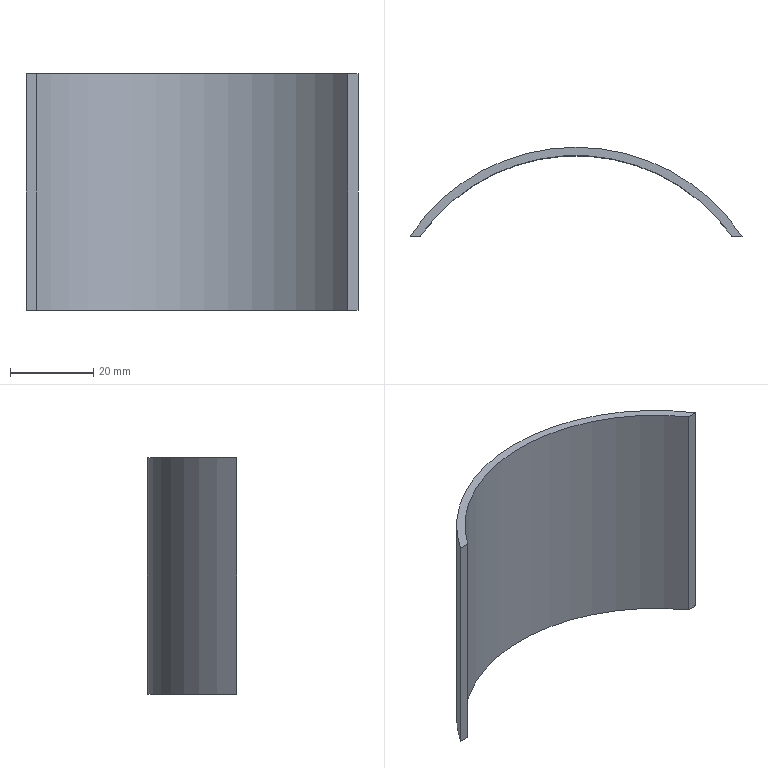Part | SolidWorks | features Extrusion 1 | 1 solid | 6 faces | box 80 x 21.467 x 57 mm | volume 10404 mm3 | plane 4 | cylinder 2 | commonest cylinder face diameters 92 x1 96 x1
STEP:
#1=CARTESIAN_POINT('',(40.,26.533,-28.5));
#2=VERTEX_POINT('',#1);
#3=CARTESIAN_POINT('',(-40.,26.533,-28.5));
#4=VERTEX_POINT('',#3);
#5=CARTESIAN_POINT('',(0.,0.,-28.5));
#6=DIRECTION('',(0.,0.,1.));
#7=DIRECTION('',(1.,0.,0.));
#8=AXIS2_PLACEMENT_3D('',#5,#6,#7);
#9=CIRCLE('',#8,48.);
#10=EDGE_CURVE('',#2,#4,#9,.T.);
#11=ORIENTED_EDGE('',*,*,#10,.T.);
#12=CARTESIAN_POINT('',(-40.,26.533,28.5));
#13=VERTEX_POINT('',#12);
#14=CARTESIAN_POINT('',(-40.,26.533,28.5));
#15=DIRECTION('',(0.,0.,-1.));
#16=VECTOR('',#15,1000.);
#17=LINE('',#14,#16);
#18=EDGE_CURVE('',#13,#4,#17,.T.);
#19=ORIENTED_EDGE('',*,*,#18,.F.);
#20=CARTESIAN_POINT('',(40.,26.533,28.5));
#21=VERTEX_POINT('',#20);
#22=CARTESIAN_POINT('',(0.,0.,28.5));
#23=DIRECTION('',(0.,0.,1.));
#24=DIRECTION('',(1.,0.,0.));
#25=AXIS2_PLACEMENT_3D('',#22,#23,#24);
#26=CIRCLE('',#25,48.);
#27=EDGE_CURVE('',#21,#13,#26,.T.);
#28=ORIENTED_EDGE('',*,*,#27,.F.);
#29=CARTESIAN_POINT('',(40.,26.533,28.5));
#30=DIRECTION('',(0.,0.,-1.));
#31=VECTOR('',#30,1000.);
#32=LINE('',#29,#31);
#33=EDGE_CURVE('',#21,#2,#32,.T.);
#34=ORIENTED_EDGE('',*,*,#33,.T.);
#35=EDGE_LOOP('',(#11,#19,#28,#34));
#36=FACE_OUTER_BOUND('',#35,.T.);
#37=CARTESIAN_POINT('',(0.,0.,28.5));
#38=DIRECTION('',(0.,0.,-1.));
#39=DIRECTION('',(-1.,0.,0.));
#40=AXIS2_PLACEMENT_3D('',#37,#38,#39);
#41=CYLINDRICAL_SURFACE('',#40,48.);
#42=ADVANCED_FACE('',(#36),#41,.T.);
#43=CARTESIAN_POINT('',(-37.577,26.533,-28.5));
#44=VERTEX_POINT('',#43);
#45=CARTESIAN_POINT('',(-40.,26.533,-28.5));
#46=DIRECTION('',(1.,0.,0.));
#47=VECTOR('',#46,1000.);
#48=LINE('',#45,#47);
#49=EDGE_CURVE('',#4,#44,#48,.T.);
#50=ORIENTED_EDGE('',*,*,#49,.T.);
#51=CARTESIAN_POINT('',(-37.577,26.533,28.5));
#52=VERTEX_POINT('',#51);
#53=CARTESIAN_POINT('',(-37.577,26.533,28.5));
#54=DIRECTION('',(0.,0.,-1.));
#55=VECTOR('',#54,1000.);
#56=LINE('',#53,#55);
#57=EDGE_CURVE('',#52,#44,#56,.T.);
#58=ORIENTED_EDGE('',*,*,#57,.F.);
#59=CARTESIAN_POINT('',(-40.,26.533,28.5));
#60=DIRECTION('',(1.,0.,0.));
#61=VECTOR('',#60,1000.);
#62=LINE('',#59,#61);
#63=EDGE_CURVE('',#13,#52,#62,.T.);
#64=ORIENTED_EDGE('',*,*,#63,.F.);
#65=ORIENTED_EDGE('',*,*,#18,.T.);
#66=EDGE_LOOP('',(#50,#58,#64,#65));
#67=FACE_OUTER_BOUND('',#66,.T.);
#68=CARTESIAN_POINT('',(-40.,26.533,28.5));
#69=DIRECTION('',(0.,1.,0.));
#70=DIRECTION('',(0.,0.,1.));
#71=AXIS2_PLACEMENT_3D('',#68,#69,#70);
#72=PLANE('',#71);
#73=ADVANCED_FACE('',(#67),#72,.F.);
#74=CARTESIAN_POINT('',(37.577,26.533,-28.5));
#75=VERTEX_POINT('',#74);
#76=CARTESIAN_POINT('',(0.,0.,-28.5));
#77=DIRECTION('',(0.,0.,-1.));
#78=DIRECTION('',(1.,0.,0.));
#79=AXIS2_PLACEMENT_3D('',#76,#77,#78);
#80=CIRCLE('',#79,46.);
#81=EDGE_CURVE('',#44,#75,#80,.T.);
#82=ORIENTED_EDGE('',*,*,#81,.T.);
#83=CARTESIAN_POINT('',(37.577,26.533,28.5));
#84=VERTEX_POINT('',#83);
#85=CARTESIAN_POINT('',(37.577,26.533,28.5));
#86=DIRECTION('',(0.,0.,-1.));
#87=VECTOR('',#86,1000.);
#88=LINE('',#85,#87);
#89=EDGE_CURVE('',#84,#75,#88,.T.);
#90=ORIENTED_EDGE('',*,*,#89,.F.);
#91=CARTESIAN_POINT('',(0.,0.,28.5));
#92=DIRECTION('',(0.,0.,-1.));
#93=DIRECTION('',(1.,0.,0.));
#94=AXIS2_PLACEMENT_3D('',#91,#92,#93);
#95=CIRCLE('',#94,46.);
#96=EDGE_CURVE('',#52,#84,#95,.T.);
#97=ORIENTED_EDGE('',*,*,#96,.F.);
#98=ORIENTED_EDGE('',*,*,#57,.T.);
#99=EDGE_LOOP('',(#82,#90,#97,#98));
#100=FACE_OUTER_BOUND('',#99,.T.);
#101=CARTESIAN_POINT('',(0.,0.,28.5));
#102=DIRECTION('',(0.,0.,-1.));
#103=DIRECTION('',(-1.,0.,0.));
#104=AXIS2_PLACEMENT_3D('',#101,#102,#103);
#105=CYLINDRICAL_SURFACE('',#104,46.);
#106=ADVANCED_FACE('',(#100),#105,.F.);
#107=CARTESIAN_POINT('',(37.577,26.533,-28.5));
#108=DIRECTION('',(1.,0.,0.));
#109=VECTOR('',#108,1000.);
#110=LINE('',#107,#109);
#111=EDGE_CURVE('',#75,#2,#110,.T.);
#112=ORIENTED_EDGE('',*,*,#111,.T.);
#113=ORIENTED_EDGE('',*,*,#33,.F.);
#114=CARTESIAN_POINT('',(37.577,26.533,28.5));
#115=DIRECTION('',(1.,0.,0.));
#116=VECTOR('',#115,1000.);
#117=LINE('',#114,#116);
#118=EDGE_CURVE('',#84,#21,#117,.T.);
#119=ORIENTED_EDGE('',*,*,#118,.F.);
#120=ORIENTED_EDGE('',*,*,#89,.T.);
#121=EDGE_LOOP('',(#112,#113,#119,#120));
#122=FACE_OUTER_BOUND('',#121,.T.);
#123=CARTESIAN_POINT('',(37.577,26.533,28.5));
#124=DIRECTION('',(0.,1.,0.));
#125=DIRECTION('',(0.,0.,1.));
#126=AXIS2_PLACEMENT_3D('',#123,#124,#125);
#127=PLANE('',#126);
#128=ADVANCED_FACE('',(#122),#127,.F.);
#129=ORIENTED_EDGE('',*,*,#27,.T.);
#130=ORIENTED_EDGE('',*,*,#63,.T.);
#131=ORIENTED_EDGE('',*,*,#96,.T.);
#132=ORIENTED_EDGE('',*,*,#118,.T.);
#133=EDGE_LOOP('',(#129,#130,#131,#132));
#134=FACE_OUTER_BOUND('',#133,.T.);
#135=CARTESIAN_POINT('',(0.,0.,28.5));
#136=DIRECTION('',(0.,0.,1.));
#137=DIRECTION('',(1.,0.,0.));
#138=AXIS2_PLACEMENT_3D('',#135,#136,#137);
#139=PLANE('',#138);
#140=ADVANCED_FACE('',(#134),#139,.T.);
#141=ORIENTED_EDGE('',*,*,#10,.F.);
#142=ORIENTED_EDGE('',*,*,#111,.F.);
#143=ORIENTED_EDGE('',*,*,#81,.F.);
#144=ORIENTED_EDGE('',*,*,#49,.F.);
#145=EDGE_LOOP('',(#141,#142,#143,#144));
#146=FACE_OUTER_BOUND('',#145,.T.);
#147=CARTESIAN_POINT('',(0.,0.,-28.5));
#148=DIRECTION('',(0.,0.,1.));
#149=DIRECTION('',(1.,0.,0.));
#150=AXIS2_PLACEMENT_3D('',#147,#148,#149);
#151=PLANE('',#150);
#152=ADVANCED_FACE('',(#146),#151,.F.);
#153=CLOSED_SHELL('',(#42,#73,#106,#128,#140,#152));
#154=MANIFOLD_SOLID_BREP('',#153);
#155=CARTESIAN_POINT('',(0.,0.,0.));
#156=DIRECTION('',(0.,0.,1.));
#157=DIRECTION('',(1.,0.,0.));
#158=AXIS2_PLACEMENT_3D('',#155,#156,#157);
#159=(LENGTH_UNIT()NAMED_UNIT(*)SI_UNIT(.MILLI.,.METRE.));
#160=UNCERTAINTY_MEASURE_WITH_UNIT(LENGTH_MEASURE(0.00001),#159,'','');
#161=(NAMED_UNIT(*)PLANE_ANGLE_UNIT()SI_UNIT($,.RADIAN.));
#162=(NAMED_UNIT(*)SI_UNIT($,.STERADIAN.)SOLID_ANGLE_UNIT());
#163=(GEOMETRIC_REPRESENTATION_CONTEXT(3)GLOBAL_UNCERTAINTY_ASSIGNED_CONTEXT((#160))GLOBAL_UNIT_ASSIGNED_CONTEXT((#159,#161,#162))REPRESENTATION_CONTEXT('',''));
#164=ADVANCED_BREP_SHAPE_REPRESENTATION('',(#154,#158),#163);